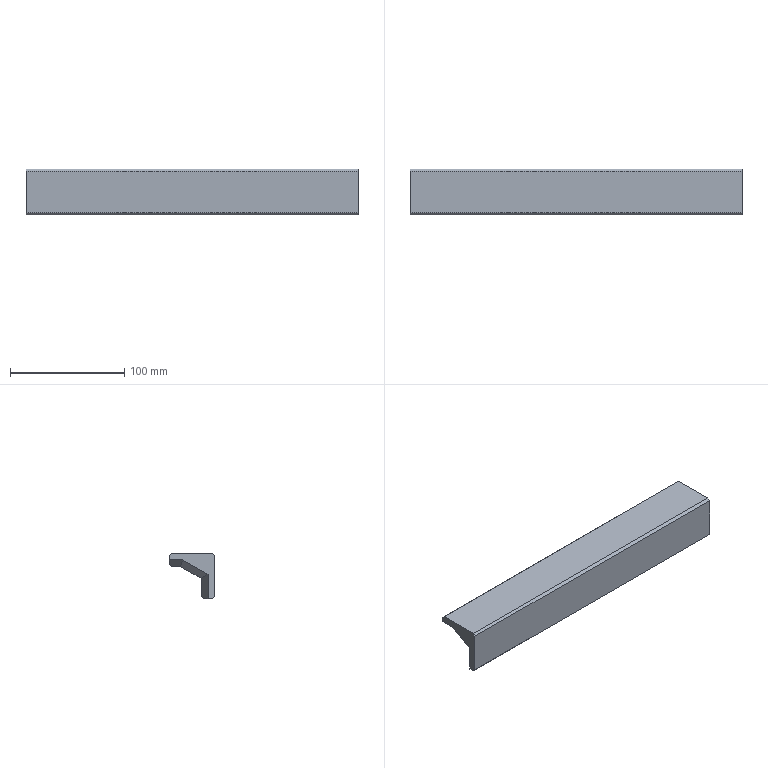Part | NX | 1 solid | 25 faces | box 290 x 40 x 40 mm | volume 257462 mm3 | plane 17 | cone 4 | cylinder 4 | commonest cylinder face diameters 4.2 x4
STEP:
#1=CARTESIAN_POINT('',(145.,-18.,20.));
#2=VERTEX_POINT('',#1);
#3=CARTESIAN_POINT('',(145.,-20.,18.));
#4=VERTEX_POINT('',#3);
#5=CARTESIAN_POINT('',(145.,-19.,19.));
#6=DIRECTION('',(0.,-0.7071,-0.7071));
#7=VECTOR('',#6,1000.);
#8=LINE('',#5,#7);
#9=EDGE_CURVE('',#2,#4,#8,.T.);
#10=ORIENTED_EDGE('',*,*,#9,.F.);
#11=CARTESIAN_POINT('',(-145.,-18.,20.));
#12=VERTEX_POINT('',#11);
#13=CARTESIAN_POINT('',(145.,-18.,20.));
#14=DIRECTION('',(1.,0.,0.));
#15=VECTOR('',#14,1000.);
#16=LINE('',#13,#15);
#17=EDGE_CURVE('',#12,#2,#16,.T.);
#18=ORIENTED_EDGE('',*,*,#17,.F.);
#19=CARTESIAN_POINT('',(-145.,-20.,18.));
#20=VERTEX_POINT('',#19);
#21=CARTESIAN_POINT('',(-145.,-20.,18.));
#22=DIRECTION('',(0.,0.7071,0.7071));
#23=VECTOR('',#22,1000.);
#24=LINE('',#21,#23);
#25=EDGE_CURVE('',#20,#12,#24,.T.);
#26=ORIENTED_EDGE('',*,*,#25,.F.);
#27=CARTESIAN_POINT('',(145.,-20.,18.));
#28=DIRECTION('',(-1.,0.,0.));
#29=VECTOR('',#28,1000.);
#30=LINE('',#27,#29);
#31=EDGE_CURVE('',#4,#20,#30,.T.);
#32=ORIENTED_EDGE('',*,*,#31,.F.);
#33=EDGE_LOOP('',(#10,#18,#26,#32));
#34=FACE_BOUND('',#33,.T.);
#35=CARTESIAN_POINT('',(145.,-20.,18.));
#36=DIRECTION('',(0.,0.7071,-0.7071));
#37=DIRECTION('',(-1.,0.,0.));
#38=AXIS2_PLACEMENT_3D('',#35,#36,#37);
#39=PLANE('',#38);
#40=ADVANCED_FACE('',(#34),#39,.F.);
#41=CARTESIAN_POINT('',(145.,-20.,-18.));
#42=VERTEX_POINT('',#41);
#43=CARTESIAN_POINT('',(145.,-18.,-20.));
#44=VERTEX_POINT('',#43);
#45=CARTESIAN_POINT('',(145.,-19.,-19.));
#46=DIRECTION('',(0.,0.7071,-0.7071));
#47=VECTOR('',#46,1000.);
#48=LINE('',#45,#47);
#49=EDGE_CURVE('',#42,#44,#48,.T.);
#50=ORIENTED_EDGE('',*,*,#49,.F.);
#51=CARTESIAN_POINT('',(-145.,-20.,-18.));
#52=VERTEX_POINT('',#51);
#53=CARTESIAN_POINT('',(145.,-20.,-18.));
#54=DIRECTION('',(1.,0.,0.));
#55=VECTOR('',#54,1000.);
#56=LINE('',#53,#55);
#57=EDGE_CURVE('',#52,#42,#56,.T.);
#58=ORIENTED_EDGE('',*,*,#57,.F.);
#59=CARTESIAN_POINT('',(-145.,-18.,-20.));
#60=VERTEX_POINT('',#59);
#61=CARTESIAN_POINT('',(-145.,-18.,-20.));
#62=DIRECTION('',(0.,-0.7071,0.7071));
#63=VECTOR('',#62,1000.);
#64=LINE('',#61,#63);
#65=EDGE_CURVE('',#60,#52,#64,.T.);
#66=ORIENTED_EDGE('',*,*,#65,.F.);
#67=CARTESIAN_POINT('',(145.,-18.,-20.));
#68=DIRECTION('',(-1.,0.,0.));
#69=VECTOR('',#68,1000.);
#70=LINE('',#67,#69);
#71=EDGE_CURVE('',#44,#60,#70,.T.);
#72=ORIENTED_EDGE('',*,*,#71,.F.);
#73=EDGE_LOOP('',(#50,#58,#66,#72));
#74=FACE_BOUND('',#73,.T.);
#75=CARTESIAN_POINT('',(145.,-18.,-20.));
#76=DIRECTION('',(0.,0.7071,0.7071));
#77=DIRECTION('',(-1.,0.,0.));
#78=AXIS2_PLACEMENT_3D('',#75,#76,#77);
#79=PLANE('',#78);
#80=ADVANCED_FACE('',(#74),#79,.F.);
#81=CARTESIAN_POINT('',(145.,20.,18.));
#82=VERTEX_POINT('',#81);
#83=CARTESIAN_POINT('',(145.,18.,20.));
#84=VERTEX_POINT('',#83);
#85=CARTESIAN_POINT('',(145.,19.,19.));
#86=DIRECTION('',(0.,-0.7071,0.7071));
#87=VECTOR('',#86,1000.);
#88=LINE('',#85,#87);
#89=EDGE_CURVE('',#82,#84,#88,.T.);
#90=ORIENTED_EDGE('',*,*,#89,.F.);
#91=CARTESIAN_POINT('',(-145.,20.,18.));
#92=VERTEX_POINT('',#91);
#93=CARTESIAN_POINT('',(145.,20.,18.));
#94=DIRECTION('',(1.,0.,0.));
#95=VECTOR('',#94,1000.);
#96=LINE('',#93,#95);
#97=EDGE_CURVE('',#92,#82,#96,.T.);
#98=ORIENTED_EDGE('',*,*,#97,.F.);
#99=CARTESIAN_POINT('',(-145.,18.,20.));
#100=VERTEX_POINT('',#99);
#101=CARTESIAN_POINT('',(-145.,18.,20.));
#102=DIRECTION('',(0.,0.7071,-0.7071));
#103=VECTOR('',#102,1000.);
#104=LINE('',#101,#103);
#105=EDGE_CURVE('',#100,#92,#104,.T.);
#106=ORIENTED_EDGE('',*,*,#105,.F.);
#107=CARTESIAN_POINT('',(145.,18.,20.));
#108=DIRECTION('',(-1.,0.,0.));
#109=VECTOR('',#108,1000.);
#110=LINE('',#107,#109);
#111=EDGE_CURVE('',#84,#100,#110,.T.);
#112=ORIENTED_EDGE('',*,*,#111,.F.);
#113=EDGE_LOOP('',(#90,#98,#106,#112));
#114=FACE_BOUND('',#113,.T.);
#115=CARTESIAN_POINT('',(145.,18.,20.));
#116=DIRECTION('',(0.,-0.7071,-0.7071));
#117=DIRECTION('',(-1.,0.,0.));
#118=AXIS2_PLACEMENT_3D('',#115,#116,#117);
#119=PLANE('',#118);
#120=ADVANCED_FACE('',(#114),#119,.F.);
#121=CARTESIAN_POINT('',(-138.333,20.,10.));
#122=VERTEX_POINT('',#121);
#123=CARTESIAN_POINT('',(-135.,18.,8.));
#124=VERTEX_POINT('',#123);
#125=CARTESIAN_POINT('',(-136.628,18.977,8.977));
#126=DIRECTION('',(0.7625,-0.4575,-0.4575));
#127=VECTOR('',#126,1000.);
#128=LINE('',#125,#127);
#129=EDGE_CURVE('',#122,#124,#128,.T.);
#130=ORIENTED_EDGE('',*,*,#129,.F.);
#131=CARTESIAN_POINT('',(145.,20.,10.));
#132=VERTEX_POINT('',#131);
#133=CARTESIAN_POINT('',(145.,20.,10.));
#134=DIRECTION('',(-1.,0.,0.));
#135=VECTOR('',#134,1000.);
#136=LINE('',#133,#135);
#137=EDGE_CURVE('',#132,#122,#136,.T.);
#138=ORIENTED_EDGE('',*,*,#137,.F.);
#139=CARTESIAN_POINT('',(145.,18.,8.));
#140=VERTEX_POINT('',#139);
#141=CARTESIAN_POINT('',(145.,5.,-5.));
#142=DIRECTION('',(0.,0.7071,0.7071));
#143=VECTOR('',#142,1000.);
#144=LINE('',#141,#143);
#145=EDGE_CURVE('',#140,#132,#144,.T.);
#146=ORIENTED_EDGE('',*,*,#145,.F.);
#147=CARTESIAN_POINT('',(-145.,18.,8.));
#148=DIRECTION('',(1.,0.,0.));
#149=VECTOR('',#148,1000.);
#150=LINE('',#147,#149);
#151=EDGE_CURVE('',#124,#140,#150,.T.);
#152=ORIENTED_EDGE('',*,*,#151,.F.);
#153=EDGE_LOOP('',(#130,#138,#146,#152));
#154=FACE_BOUND('',#153,.T.);
#155=CARTESIAN_POINT('',(145.,-10.,-20.));
#156=DIRECTION('',(0.,-0.7071,0.7071));
#157=DIRECTION('',(1.,0.,0.));
#158=AXIS2_PLACEMENT_3D('',#155,#156,#157);
#159=PLANE('',#158);
#160=ADVANCED_FACE('',(#154),#159,.F.);
#161=CARTESIAN_POINT('',(-135.,-8.,-18.));
#162=VERTEX_POINT('',#161);
#163=CARTESIAN_POINT('',(-138.333,-10.,-20.));
#164=VERTEX_POINT('',#163);
#165=CARTESIAN_POINT('',(-136.628,-8.977,-18.977));
#166=DIRECTION('',(-0.7625,-0.4575,-0.4575));
#167=VECTOR('',#166,1000.);
#168=LINE('',#165,#167);
#169=EDGE_CURVE('',#162,#164,#168,.T.);
#170=ORIENTED_EDGE('',*,*,#169,.F.);
#171=CARTESIAN_POINT('',(145.,-8.,-18.));
#172=VERTEX_POINT('',#171);
#173=CARTESIAN_POINT('',(-145.,-8.,-18.));
#174=DIRECTION('',(-1.,0.,0.));
#175=VECTOR('',#174,1000.);
#176=LINE('',#173,#175);
#177=EDGE_CURVE('',#172,#162,#176,.T.);
#178=ORIENTED_EDGE('',*,*,#177,.F.);
#179=CARTESIAN_POINT('',(145.,-10.,-20.));
#180=VERTEX_POINT('',#179);
#181=CARTESIAN_POINT('',(145.,5.,-5.));
#182=DIRECTION('',(0.,0.7071,0.7071));
#183=VECTOR('',#182,1000.);
#184=LINE('',#181,#183);
#185=EDGE_CURVE('',#180,#172,#184,.T.);
#186=ORIENTED_EDGE('',*,*,#185,.F.);
#187=CARTESIAN_POINT('',(145.,-10.,-20.));
#188=DIRECTION('',(1.,0.,0.));
#189=VECTOR('',#188,1000.);
#190=LINE('',#187,#189);
#191=EDGE_CURVE('',#164,#180,#190,.T.);
#192=ORIENTED_EDGE('',*,*,#191,.F.);
#193=EDGE_LOOP('',(#170,#178,#186,#192));
#194=FACE_BOUND('',#193,.T.);
#195=CARTESIAN_POINT('',(145.,-10.,-20.));
#196=DIRECTION('',(0.,-0.7071,0.7071));
#197=DIRECTION('',(1.,0.,0.));
#198=AXIS2_PLACEMENT_3D('',#195,#196,#197);
#199=PLANE('',#198);
#200=ADVANCED_FACE('',(#194),#199,.F.);
#201=CARTESIAN_POINT('',(-135.,-8.,-2.));
#202=VERTEX_POINT('',#201);
#203=CARTESIAN_POINT('',(-135.,-8.,-20.));
#204=DIRECTION('',(0.,0.,1.));
#205=VECTOR('',#204,1000.);
#206=LINE('',#203,#205);
#207=EDGE_CURVE('',#162,#202,#206,.T.);
#208=ORIENTED_EDGE('',*,*,#207,.F.);
#209=ORIENTED_EDGE('',*,*,#169,.T.);
#210=CARTESIAN_POINT('',(-145.,-14.,-20.));
#211=VERTEX_POINT('',#210);
#212=CARTESIAN_POINT('',(-145.,-14.,-20.));
#213=DIRECTION('',(0.8575,0.5145,0.));
#214=VECTOR('',#213,1000.);
#215=LINE('',#212,#214);
#216=EDGE_CURVE('',#211,#164,#215,.T.);
#217=ORIENTED_EDGE('',*,*,#216,.F.);
#218=CARTESIAN_POINT('',(-145.,-14.,1.53));
#219=VERTEX_POINT('',#218);
#220=CARTESIAN_POINT('',(-145.,-14.,0.));
#221=DIRECTION('',(0.,0.,-1.));
#222=VECTOR('',#221,1000.);
#223=LINE('',#220,#222);
#224=EDGE_CURVE('',#219,#211,#223,.T.);
#225=ORIENTED_EDGE('',*,*,#224,.F.);
#226=CARTESIAN_POINT('',(-144.636,-13.782,1.402));
#227=DIRECTION('',(0.8207,0.4924,-0.2897));
#228=VECTOR('',#227,1000.);
#229=LINE('',#226,#228);
#230=EDGE_CURVE('',#219,#202,#229,.T.);
#231=ORIENTED_EDGE('',*,*,#230,.T.);
#232=EDGE_LOOP('',(#208,#209,#217,#225,#231));
#233=FACE_BOUND('',#232,.T.);
#234=CARTESIAN_POINT('',(-145.,-14.,0.));
#235=DIRECTION('',(0.5145,-0.8575,0.));
#236=DIRECTION('',(0.,0.,-1.));
#237=AXIS2_PLACEMENT_3D('',#234,#235,#236);
#238=PLANE('',#237);
#239=ADVANCED_FACE('',(#233),#238,.F.);
#240=CARTESIAN_POINT('',(-145.,8.445,14.));
#241=VERTEX_POINT('',#240);
#242=CARTESIAN_POINT('',(-135.,10.,8.));
#243=VERTEX_POINT('',#242);
#244=CARTESIAN_POINT('',(-143.407,8.693,13.044));
#245=DIRECTION('',(0.85,0.1321,-0.51));
#246=VECTOR('',#245,1000.);
#247=LINE('',#244,#246);
#248=EDGE_CURVE('',#241,#243,#247,.T.);
#249=ORIENTED_EDGE('',*,*,#248,.T.);
#250=CARTESIAN_POINT('',(-135.,-8.,-2.));
#251=DIRECTION('',(0.,0.8742,0.4856));
#252=VECTOR('',#251,1000.);
#253=LINE('',#250,#252);
#254=EDGE_CURVE('',#202,#243,#253,.T.);
#255=ORIENTED_EDGE('',*,*,#254,.F.);
#256=ORIENTED_EDGE('',*,*,#230,.F.);
#257=CARTESIAN_POINT('',(-145.,-3.952,7.113));
#258=DIRECTION('',(0.,-0.8742,-0.4856));
#259=VECTOR('',#258,1000.);
#260=LINE('',#257,#259);
#261=EDGE_CURVE('',#241,#219,#260,.T.);
#262=ORIENTED_EDGE('',*,*,#261,.F.);
#263=EDGE_LOOP('',(#249,#255,#256,#262));
#264=FACE_BOUND('',#263,.T.);
#265=CARTESIAN_POINT('',(-145.,-3.952,7.113));
#266=DIRECTION('',(-0.5145,0.4164,-0.7496));
#267=DIRECTION('',(0.,0.8742,0.4856));
#268=AXIS2_PLACEMENT_3D('',#265,#266,#267);
#269=PLANE('',#268);
#270=ADVANCED_FACE('',(#264),#269,.T.);
#271=CARTESIAN_POINT('',(-145.,20.,14.));
#272=VERTEX_POINT('',#271);
#273=CARTESIAN_POINT('',(-145.,20.,14.));
#274=DIRECTION('',(-0.8575,0.,0.5145));
#275=VECTOR('',#274,1000.);
#276=LINE('',#273,#275);
#277=EDGE_CURVE('',#122,#272,#276,.T.);
#278=ORIENTED_EDGE('',*,*,#277,.F.);
#279=ORIENTED_EDGE('',*,*,#129,.T.);
#280=CARTESIAN_POINT('',(-135.,20.,8.));
#281=DIRECTION('',(0.,1.,0.));
#282=VECTOR('',#281,1000.);
#283=LINE('',#280,#282);
#284=EDGE_CURVE('',#243,#124,#283,.T.);
#285=ORIENTED_EDGE('',*,*,#284,.F.);
#286=ORIENTED_EDGE('',*,*,#248,.F.);
#287=CARTESIAN_POINT('',(-145.,0.,14.));
#288=DIRECTION('',(0.,-1.,0.));
#289=VECTOR('',#288,1000.);
#290=LINE('',#287,#289);
#291=EDGE_CURVE('',#272,#241,#290,.T.);
#292=ORIENTED_EDGE('',*,*,#291,.F.);
#293=EDGE_LOOP('',(#278,#279,#285,#286,#292));
#294=FACE_BOUND('',#293,.T.);
#295=CARTESIAN_POINT('',(-145.,0.,14.));
#296=DIRECTION('',(0.5145,0.,0.8575));
#297=DIRECTION('',(0.,-1.,0.));
#298=AXIS2_PLACEMENT_3D('',#295,#296,#297);
#299=PLANE('',#298);
#300=ADVANCED_FACE('',(#294),#299,.F.);
#301=CARTESIAN_POINT('',(145.,-8.,-2.));
#302=VERTEX_POINT('',#301);
#303=CARTESIAN_POINT('',(145.,-8.,-2.));
#304=DIRECTION('',(1.,0.,0.));
#305=VECTOR('',#304,1000.);
#306=LINE('',#303,#305);
#307=EDGE_CURVE('',#202,#302,#306,.T.);
#308=ORIENTED_EDGE('',*,*,#307,.F.);
#309=ORIENTED_EDGE('',*,*,#254,.T.);
#310=CARTESIAN_POINT('',(145.,10.,8.));
#311=VERTEX_POINT('',#310);
#312=CARTESIAN_POINT('',(-145.,10.,8.));
#313=DIRECTION('',(-1.,0.,0.));
#314=VECTOR('',#313,1000.);
#315=LINE('',#312,#314);
#316=EDGE_CURVE('',#311,#243,#315,.T.);
#317=ORIENTED_EDGE('',*,*,#316,.F.);
#318=CARTESIAN_POINT('',(145.,-8.,-2.));
#319=DIRECTION('',(0.,0.8742,0.4856));
#320=VECTOR('',#319,1000.);
#321=LINE('',#318,#320);
#322=EDGE_CURVE('',#302,#311,#321,.T.);
#323=ORIENTED_EDGE('',*,*,#322,.F.);
#324=EDGE_LOOP('',(#308,#309,#317,#323));
#325=FACE_BOUND('',#324,.T.);
#326=CARTESIAN_POINT('',(-145.,-8.,-2.));
#327=DIRECTION('',(0.,0.4856,-0.8742));
#328=DIRECTION('',(-1.,0.,0.));
#329=AXIS2_PLACEMENT_3D('',#326,#327,#328);
#330=PLANE('',#329);
#331=ADVANCED_FACE('',(#325),#330,.T.);
#332=ORIENTED_EDGE('',*,*,#284,.T.);
#333=ORIENTED_EDGE('',*,*,#151,.T.);
#334=CARTESIAN_POINT('',(145.,20.,8.));
#335=DIRECTION('',(0.,-1.,0.));
#336=VECTOR('',#335,1000.);
#337=LINE('',#334,#336);
#338=EDGE_CURVE('',#140,#311,#337,.T.);
#339=ORIENTED_EDGE('',*,*,#338,.T.);
#340=ORIENTED_EDGE('',*,*,#316,.T.);
#341=EDGE_LOOP('',(#332,#333,#339,#340));
#342=FACE_BOUND('',#341,.T.);
#343=CARTESIAN_POINT('',(-145.,20.,8.));
#344=DIRECTION('',(0.,0.,1.));
#345=DIRECTION('',(0.,-1.,0.));
#346=AXIS2_PLACEMENT_3D('',#343,#344,#345);
#347=PLANE('',#346);
#348=ADVANCED_FACE('',(#342),#347,.F.);
#349=CARTESIAN_POINT('',(145.,-8.,-20.));
#350=DIRECTION('',(0.,0.,-1.));
#351=VECTOR('',#350,1000.);
#352=LINE('',#349,#351);
#353=EDGE_CURVE('',#302,#172,#352,.T.);
#354=ORIENTED_EDGE('',*,*,#353,.T.);
#355=ORIENTED_EDGE('',*,*,#177,.T.);
#356=ORIENTED_EDGE('',*,*,#207,.T.);
#357=ORIENTED_EDGE('',*,*,#307,.T.);
#358=EDGE_LOOP('',(#354,#355,#356,#357));
#359=FACE_BOUND('',#358,.T.);
#360=CARTESIAN_POINT('',(-145.,-8.,-20.));
#361=DIRECTION('',(0.,-1.,0.));
#362=DIRECTION('',(0.,0.,-1.));
#363=AXIS2_PLACEMENT_3D('',#360,#361,#362);
#364=PLANE('',#363);
#365=ADVANCED_FACE('',(#359),#364,.F.);
#366=CARTESIAN_POINT('',(-145.,20.,20.));
#367=DIRECTION('',(0.,-1.,0.));
#368=VECTOR('',#367,1000.);
#369=LINE('',#366,#368);
#370=EDGE_CURVE('',#100,#12,#369,.T.);
#371=ORIENTED_EDGE('',*,*,#370,.F.);
#372=ORIENTED_EDGE('',*,*,#105,.T.);
#373=CARTESIAN_POINT('',(-145.,20.,20.));
#374=DIRECTION('',(0.,0.,1.));
#375=VECTOR('',#374,1000.);
#376=LINE('',#373,#375);
#377=EDGE_CURVE('',#272,#92,#376,.T.);
#378=ORIENTED_EDGE('',*,*,#377,.F.);
#379=ORIENTED_EDGE('',*,*,#291,.T.);
#380=ORIENTED_EDGE('',*,*,#261,.T.);
#381=ORIENTED_EDGE('',*,*,#224,.T.);
#382=CARTESIAN_POINT('',(-145.,20.,-20.));
#383=DIRECTION('',(0.,1.,0.));
#384=VECTOR('',#383,1000.);
#385=LINE('',#382,#384);
#386=EDGE_CURVE('',#60,#211,#385,.T.);
#387=ORIENTED_EDGE('',*,*,#386,.F.);
#388=ORIENTED_EDGE('',*,*,#65,.T.);
#389=CARTESIAN_POINT('',(-145.,-20.,20.));
#390=DIRECTION('',(0.,0.,-1.));
#391=VECTOR('',#390,1000.);
#392=LINE('',#389,#391);
#393=EDGE_CURVE('',#20,#52,#392,.T.);
#394=ORIENTED_EDGE('',*,*,#393,.F.);
#395=ORIENTED_EDGE('',*,*,#25,.T.);
#396=EDGE_LOOP('',(#371,#372,#378,#379,#380,#381,#387,#388,#394,#395));
#397=FACE_BOUND('',#396,.T.);
#398=CARTESIAN_POINT('',(-145.,0.,0.));
#399=DIRECTION('',(1.,0.,0.));
#400=DIRECTION('',(0.,0.,-1.));
#401=AXIS2_PLACEMENT_3D('',#398,#399,#400);
#402=PLANE('',#401);
#403=ADVANCED_FACE('',(#397),#402,.F.);
#404=CARTESIAN_POINT('',(145.,20.,-20.));
#405=DIRECTION('',(0.,1.,0.));
#406=VECTOR('',#405,1000.);
#407=LINE('',#404,#406);
#408=EDGE_CURVE('',#44,#180,#407,.T.);
#409=ORIENTED_EDGE('',*,*,#408,.T.);
#410=ORIENTED_EDGE('',*,*,#185,.T.);
#411=ORIENTED_EDGE('',*,*,#353,.F.);
#412=ORIENTED_EDGE('',*,*,#322,.T.);
#413=ORIENTED_EDGE('',*,*,#338,.F.);
#414=ORIENTED_EDGE('',*,*,#145,.T.);
#415=CARTESIAN_POINT('',(145.,20.,20.));
#416=DIRECTION('',(0.,0.,1.));
#417=VECTOR('',#416,1000.);
#418=LINE('',#415,#417);
#419=EDGE_CURVE('',#132,#82,#418,.T.);
#420=ORIENTED_EDGE('',*,*,#419,.T.);
#421=ORIENTED_EDGE('',*,*,#89,.T.);
#422=CARTESIAN_POINT('',(145.,20.,20.));
#423=DIRECTION('',(0.,-1.,0.));
#424=VECTOR('',#423,1000.);
#425=LINE('',#422,#424);
#426=EDGE_CURVE('',#84,#2,#425,.T.);
#427=ORIENTED_EDGE('',*,*,#426,.T.);
#428=ORIENTED_EDGE('',*,*,#9,.T.);
#429=CARTESIAN_POINT('',(145.,-20.,20.));
#430=DIRECTION('',(0.,0.,-1.));
#431=VECTOR('',#430,1000.);
#432=LINE('',#429,#431);
#433=EDGE_CURVE('',#4,#42,#432,.T.);
#434=ORIENTED_EDGE('',*,*,#433,.T.);
#435=ORIENTED_EDGE('',*,*,#49,.T.);
#436=EDGE_LOOP('',(#409,#410,#411,#412,#413,#414,#420,#421,#427,#428,#434,#435));
#437=FACE_BOUND('',#436,.T.);
#438=CARTESIAN_POINT('',(145.,-14.,-16.1));
#439=VERTEX_POINT('',#438);
#440=CARTESIAN_POINT('',(145.,-14.,-14.));
#441=DIRECTION('',(1.,0.,0.));
#442=DIRECTION('',(0.,0.,-1.));
#443=AXIS2_PLACEMENT_3D('',#440,#441,#442);
#444=CIRCLE('',#443,2.1);
#445=EDGE_CURVE('',#439,#439,#444,.T.);
#446=ORIENTED_EDGE('',*,*,#445,.F.);
#447=EDGE_LOOP('',(#446));
#448=FACE_BOUND('',#447,.T.);
#449=CARTESIAN_POINT('',(145.,-14.,-0.1));
#450=VERTEX_POINT('',#449);
#451=CARTESIAN_POINT('',(145.,-14.,2.));
#452=DIRECTION('',(1.,0.,0.));
#453=DIRECTION('',(0.,0.,-1.));
#454=AXIS2_PLACEMENT_3D('',#451,#452,#453);
#455=CIRCLE('',#454,2.1);
#456=EDGE_CURVE('',#450,#450,#455,.T.);
#457=ORIENTED_EDGE('',*,*,#456,.F.);
#458=EDGE_LOOP('',(#457));
#459=FACE_BOUND('',#458,.T.);
#460=CARTESIAN_POINT('',(145.,-2.,11.9));
#461=VERTEX_POINT('',#460);
#462=CARTESIAN_POINT('',(145.,-2.,14.));
#463=DIRECTION('',(1.,0.,0.));
#464=DIRECTION('',(0.,0.,-1.));
#465=AXIS2_PLACEMENT_3D('',#462,#463,#464);
#466=CIRCLE('',#465,2.1);
#467=EDGE_CURVE('',#461,#461,#466,.T.);
#468=ORIENTED_EDGE('',*,*,#467,.F.);
#469=EDGE_LOOP('',(#468));
#470=FACE_BOUND('',#469,.T.);
#471=CARTESIAN_POINT('',(145.,14.,11.9));
#472=VERTEX_POINT('',#471);
#473=CARTESIAN_POINT('',(145.,14.,14.));
#474=DIRECTION('',(1.,0.,0.));
#475=DIRECTION('',(0.,0.,-1.));
#476=AXIS2_PLACEMENT_3D('',#473,#474,#475);
#477=CIRCLE('',#476,2.1);
#478=EDGE_CURVE('',#472,#472,#477,.T.);
#479=ORIENTED_EDGE('',*,*,#478,.F.);
#480=EDGE_LOOP('',(#479));
#481=FACE_BOUND('',#480,.T.);
#482=CARTESIAN_POINT('',(145.,0.,0.));
#483=DIRECTION('',(1.,0.,0.));
#484=DIRECTION('',(0.,0.,-1.));
#485=AXIS2_PLACEMENT_3D('',#482,#483,#484);
#486=PLANE('',#485);
#487=ADVANCED_FACE('',(#437,#448,#459,#470,#481),#486,.T.);
#488=ORIENTED_EDGE('',*,*,#393,.T.);
#489=ORIENTED_EDGE('',*,*,#57,.T.);
#490=ORIENTED_EDGE('',*,*,#433,.F.);
#491=ORIENTED_EDGE('',*,*,#31,.T.);
#492=EDGE_LOOP('',(#488,#489,#490,#491));
#493=FACE_BOUND('',#492,.T.);
#494=CARTESIAN_POINT('',(145.,-20.,20.));
#495=DIRECTION('',(0.,1.,0.));
#496=DIRECTION('',(0.,0.,1.));
#497=AXIS2_PLACEMENT_3D('',#494,#495,#496);
#498=PLANE('',#497);
#499=ADVANCED_FACE('',(#493),#498,.F.);
#500=ORIENTED_EDGE('',*,*,#426,.F.);
#501=ORIENTED_EDGE('',*,*,#111,.T.);
#502=ORIENTED_EDGE('',*,*,#370,.T.);
#503=ORIENTED_EDGE('',*,*,#17,.T.);
#504=EDGE_LOOP('',(#500,#501,#502,#503));
#505=FACE_BOUND('',#504,.T.);
#506=CARTESIAN_POINT('',(145.,20.,20.));
#507=DIRECTION('',(0.,0.,-1.));
#508=DIRECTION('',(0.,1.,0.));
#509=AXIS2_PLACEMENT_3D('',#506,#507,#508);
#510=PLANE('',#509);
#511=ADVANCED_FACE('',(#505),#510,.F.);
#512=ORIENTED_EDGE('',*,*,#419,.F.);
#513=ORIENTED_EDGE('',*,*,#137,.T.);
#514=ORIENTED_EDGE('',*,*,#277,.T.);
#515=ORIENTED_EDGE('',*,*,#377,.T.);
#516=ORIENTED_EDGE('',*,*,#97,.T.);
#517=EDGE_LOOP('',(#512,#513,#514,#515,#516));
#518=FACE_BOUND('',#517,.T.);
#519=CARTESIAN_POINT('',(145.,20.,20.));
#520=DIRECTION('',(0.,-1.,0.));
#521=DIRECTION('',(0.,0.,-1.));
#522=AXIS2_PLACEMENT_3D('',#519,#520,#521);
#523=PLANE('',#522);
#524=ADVANCED_FACE('',(#518),#523,.F.);
#525=ORIENTED_EDGE('',*,*,#216,.T.);
#526=ORIENTED_EDGE('',*,*,#191,.T.);
#527=ORIENTED_EDGE('',*,*,#408,.F.);
#528=ORIENTED_EDGE('',*,*,#71,.T.);
#529=ORIENTED_EDGE('',*,*,#386,.T.);
#530=EDGE_LOOP('',(#525,#526,#527,#528,#529));
#531=FACE_BOUND('',#530,.T.);
#532=CARTESIAN_POINT('',(145.,20.,-20.));
#533=DIRECTION('',(0.,0.,1.));
#534=DIRECTION('',(0.,-1.,0.));
#535=AXIS2_PLACEMENT_3D('',#532,#533,#534);
#536=PLANE('',#535);
#537=ADVANCED_FACE('',(#531),#536,.F.);
#538=CARTESIAN_POINT('',(128.738,-14.,-14.));
#539=VERTEX_POINT('',#538);
#540=VERTEX_LOOP('',#539);
#541=FACE_BOUND('',#540,.T.);
#542=CARTESIAN_POINT('',(130.,-14.,-16.1));
#543=VERTEX_POINT('',#542);
#544=CARTESIAN_POINT('',(130.,-14.,-14.));
#545=DIRECTION('',(1.,0.,0.));
#546=DIRECTION('',(0.,0.,-1.));
#547=AXIS2_PLACEMENT_3D('',#544,#545,#546);
#548=CIRCLE('',#547,2.1);
#549=EDGE_CURVE('',#543,#543,#548,.T.);
#550=ORIENTED_EDGE('',*,*,#549,.T.);
#551=EDGE_LOOP('',(#550));
#552=FACE_BOUND('',#551,.T.);
#553=CARTESIAN_POINT('',(130.,-14.,-14.));
#554=DIRECTION('',(1.,0.,0.));
#555=DIRECTION('',(0.,0.,-1.));
#556=AXIS2_PLACEMENT_3D('',#553,#554,#555);
#557=CONICAL_SURFACE('',#556,2.1,1.03);
#558=ADVANCED_FACE('',(#541,#552),#557,.F.);
#559=ORIENTED_EDGE('',*,*,#445,.T.);
#560=EDGE_LOOP('',(#559));
#561=FACE_BOUND('',#560,.T.);
#562=ORIENTED_EDGE('',*,*,#549,.F.);
#563=EDGE_LOOP('',(#562));
#564=FACE_BOUND('',#563,.T.);
#565=CARTESIAN_POINT('',(145.,-14.,-14.));
#566=DIRECTION('',(1.,0.,0.));
#567=DIRECTION('',(0.,0.,-1.));
#568=AXIS2_PLACEMENT_3D('',#565,#566,#567);
#569=CYLINDRICAL_SURFACE('',#568,2.1);
#570=ADVANCED_FACE('',(#561,#564),#569,.F.);
#571=CARTESIAN_POINT('',(128.738,-14.,2.));
#572=VERTEX_POINT('',#571);
#573=VERTEX_LOOP('',#572);
#574=FACE_BOUND('',#573,.T.);
#575=CARTESIAN_POINT('',(130.,-14.,-0.1));
#576=VERTEX_POINT('',#575);
#577=CARTESIAN_POINT('',(130.,-14.,2.));
#578=DIRECTION('',(1.,0.,0.));
#579=DIRECTION('',(0.,0.,-1.));
#580=AXIS2_PLACEMENT_3D('',#577,#578,#579);
#581=CIRCLE('',#580,2.1);
#582=EDGE_CURVE('',#576,#576,#581,.T.);
#583=ORIENTED_EDGE('',*,*,#582,.T.);
#584=EDGE_LOOP('',(#583));
#585=FACE_BOUND('',#584,.T.);
#586=CARTESIAN_POINT('',(130.,-14.,2.));
#587=DIRECTION('',(1.,0.,0.));
#588=DIRECTION('',(0.,0.,-1.));
#589=AXIS2_PLACEMENT_3D('',#586,#587,#588);
#590=CONICAL_SURFACE('',#589,2.1,1.03);
#591=ADVANCED_FACE('',(#574,#585),#590,.F.);
#592=ORIENTED_EDGE('',*,*,#456,.T.);
#593=EDGE_LOOP('',(#592));
#594=FACE_BOUND('',#593,.T.);
#595=ORIENTED_EDGE('',*,*,#582,.F.);
#596=EDGE_LOOP('',(#595));
#597=FACE_BOUND('',#596,.T.);
#598=CARTESIAN_POINT('',(145.,-14.,2.));
#599=DIRECTION('',(1.,0.,0.));
#600=DIRECTION('',(0.,0.,-1.));
#601=AXIS2_PLACEMENT_3D('',#598,#599,#600);
#602=CYLINDRICAL_SURFACE('',#601,2.1);
#603=ADVANCED_FACE('',(#594,#597),#602,.F.);
#604=CARTESIAN_POINT('',(128.738,-2.,14.));
#605=VERTEX_POINT('',#604);
#606=VERTEX_LOOP('',#605);
#607=FACE_BOUND('',#606,.T.);
#608=CARTESIAN_POINT('',(130.,-2.,11.9));
#609=VERTEX_POINT('',#608);
#610=CARTESIAN_POINT('',(130.,-2.,14.));
#611=DIRECTION('',(1.,0.,0.));
#612=DIRECTION('',(0.,0.,-1.));
#613=AXIS2_PLACEMENT_3D('',#610,#611,#612);
#614=CIRCLE('',#613,2.1);
#615=EDGE_CURVE('',#609,#609,#614,.T.);
#616=ORIENTED_EDGE('',*,*,#615,.T.);
#617=EDGE_LOOP('',(#616));
#618=FACE_BOUND('',#617,.T.);
#619=CARTESIAN_POINT('',(130.,-2.,14.));
#620=DIRECTION('',(1.,0.,0.));
#621=DIRECTION('',(0.,0.,-1.));
#622=AXIS2_PLACEMENT_3D('',#619,#620,#621);
#623=CONICAL_SURFACE('',#622,2.1,1.03);
#624=ADVANCED_FACE('',(#607,#618),#623,.F.);
#625=ORIENTED_EDGE('',*,*,#467,.T.);
#626=EDGE_LOOP('',(#625));
#627=FACE_BOUND('',#626,.T.);
#628=ORIENTED_EDGE('',*,*,#615,.F.);
#629=EDGE_LOOP('',(#628));
#630=FACE_BOUND('',#629,.T.);
#631=CARTESIAN_POINT('',(145.,-2.,14.));
#632=DIRECTION('',(1.,0.,0.));
#633=DIRECTION('',(0.,0.,-1.));
#634=AXIS2_PLACEMENT_3D('',#631,#632,#633);
#635=CYLINDRICAL_SURFACE('',#634,2.1);
#636=ADVANCED_FACE('',(#627,#630),#635,.F.);
#637=CARTESIAN_POINT('',(128.738,14.,14.));
#638=VERTEX_POINT('',#637);
#639=VERTEX_LOOP('',#638);
#640=FACE_BOUND('',#639,.T.);
#641=CARTESIAN_POINT('',(130.,14.,11.9));
#642=VERTEX_POINT('',#641);
#643=CARTESIAN_POINT('',(130.,14.,14.));
#644=DIRECTION('',(1.,0.,0.));
#645=DIRECTION('',(0.,0.,-1.));
#646=AXIS2_PLACEMENT_3D('',#643,#644,#645);
#647=CIRCLE('',#646,2.1);
#648=EDGE_CURVE('',#642,#642,#647,.T.);
#649=ORIENTED_EDGE('',*,*,#648,.T.);
#650=EDGE_LOOP('',(#649));
#651=FACE_BOUND('',#650,.T.);
#652=CARTESIAN_POINT('',(130.,14.,14.));
#653=DIRECTION('',(1.,0.,0.));
#654=DIRECTION('',(0.,0.,-1.));
#655=AXIS2_PLACEMENT_3D('',#652,#653,#654);
#656=CONICAL_SURFACE('',#655,2.1,1.03);
#657=ADVANCED_FACE('',(#640,#651),#656,.F.);
#658=ORIENTED_EDGE('',*,*,#478,.T.);
#659=EDGE_LOOP('',(#658));
#660=FACE_BOUND('',#659,.T.);
#661=ORIENTED_EDGE('',*,*,#648,.F.);
#662=EDGE_LOOP('',(#661));
#663=FACE_BOUND('',#662,.T.);
#664=CARTESIAN_POINT('',(145.,14.,14.));
#665=DIRECTION('',(1.,0.,0.));
#666=DIRECTION('',(0.,0.,-1.));
#667=AXIS2_PLACEMENT_3D('',#664,#665,#666);
#668=CYLINDRICAL_SURFACE('',#667,2.1);
#669=ADVANCED_FACE('',(#660,#663),#668,.F.);
#670=CLOSED_SHELL('',(#40,#80,#120,#160,#200,#239,#270,#300,#331,#348,#365,#403,#487,#499,#511,#524,#537,#558,#570,#591,#603,#624,#636,#657,#669));
#671=MANIFOLD_SOLID_BREP('',#670);
#672=(LENGTH_UNIT()NAMED_UNIT(*)SI_UNIT(.MILLI.,.METRE.));
#673=UNCERTAINTY_MEASURE_WITH_UNIT(LENGTH_MEASURE(0.00001),#672,'','');
#674=(NAMED_UNIT(*)PLANE_ANGLE_UNIT()SI_UNIT($,.RADIAN.));
#675=(NAMED_UNIT(*)SI_UNIT($,.STERADIAN.)SOLID_ANGLE_UNIT());
#676=(GEOMETRIC_REPRESENTATION_CONTEXT(3)GLOBAL_UNCERTAINTY_ASSIGNED_CONTEXT((#673))GLOBAL_UNIT_ASSIGNED_CONTEXT((#672,#674,#675))REPRESENTATION_CONTEXT('',''));
#677=ADVANCED_BREP_SHAPE_REPRESENTATION('',(#671),#676);